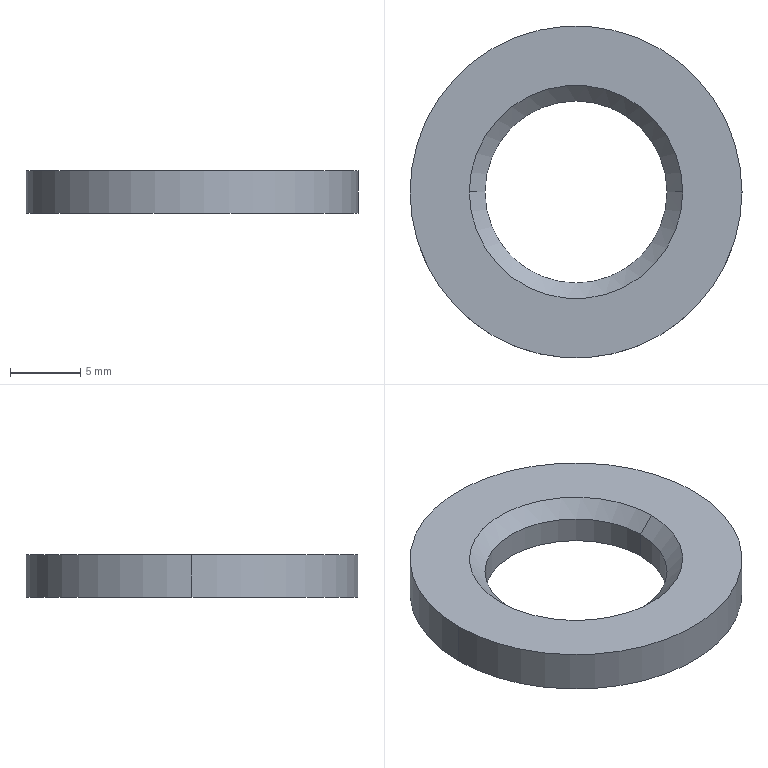Part | SolidWorks | 1 solid | 8 faces | box 23.7 x 23.7 x 3 mm | volume 898.415 mm3 | cylinder 4 | cone 2 | plane 2 | commonest cylinder face diameters 13 x2 23.7 x2
STEP:
#1=CARTESIAN_POINT('',(6.5,0.,1.885));
#2=VERTEX_POINT('',#1);
#3=CARTESIAN_POINT('',(-6.5,0.,1.885));
#4=VERTEX_POINT('',#3);
#5=CARTESIAN_POINT('',(0.,0.,1.885));
#6=DIRECTION('',(0.,0.,-1.));
#7=DIRECTION('',(1.,0.,0.));
#8=AXIS2_PLACEMENT_3D('',#5,#6,#7);
#9=CIRCLE('',#8,6.5);
#10=EDGE_CURVE('',#2,#4,#9,.T.);
#11=ORIENTED_EDGE('',*,*,#10,.T.);
#12=CARTESIAN_POINT('',(-7.615,0.,3.));
#13=VERTEX_POINT('',#12);
#14=CARTESIAN_POINT('',(-7.615,0.,3.));
#15=DIRECTION('',(-0.7071,0.,0.7071));
#16=VECTOR('',#15,1000.);
#17=LINE('',#14,#16);
#18=EDGE_CURVE('',#4,#13,#17,.T.);
#19=ORIENTED_EDGE('',*,*,#18,.T.);
#20=CARTESIAN_POINT('',(7.615,0.,3.));
#21=VERTEX_POINT('',#20);
#22=CARTESIAN_POINT('',(0.,0.,3.));
#23=DIRECTION('',(0.,0.,1.));
#24=DIRECTION('',(1.,0.,0.));
#25=AXIS2_PLACEMENT_3D('',#22,#23,#24);
#26=CIRCLE('',#25,7.615);
#27=EDGE_CURVE('',#13,#21,#26,.T.);
#28=ORIENTED_EDGE('',*,*,#27,.T.);
#29=CARTESIAN_POINT('',(7.615,0.,3.));
#30=DIRECTION('',(0.7071,0.,0.7071));
#31=VECTOR('',#30,1000.);
#32=LINE('',#29,#31);
#33=EDGE_CURVE('',#2,#21,#32,.T.);
#34=ORIENTED_EDGE('',*,*,#33,.F.);
#35=EDGE_LOOP('',(#11,#19,#28,#34));
#36=FACE_OUTER_BOUND('',#35,.T.);
#37=CARTESIAN_POINT('',(0.,0.,3.));
#38=DIRECTION('',(0.,0.,1.));
#39=DIRECTION('',(1.,0.,0.));
#40=AXIS2_PLACEMENT_3D('',#37,#38,#39);
#41=CONICAL_SURFACE('',#40,7.615,0.7854);
#42=ADVANCED_FACE('',(#36),#41,.F.);
#43=ORIENTED_EDGE('',*,*,#10,.F.);
#44=CARTESIAN_POINT('',(6.5,0.,0.));
#45=VERTEX_POINT('',#44);
#46=CARTESIAN_POINT('',(6.5,0.,3.));
#47=DIRECTION('',(0.,0.,-1.));
#48=VECTOR('',#47,1000.);
#49=LINE('',#46,#48);
#50=EDGE_CURVE('',#2,#45,#49,.T.);
#51=ORIENTED_EDGE('',*,*,#50,.T.);
#52=CARTESIAN_POINT('',(-6.5,0.,0.));
#53=VERTEX_POINT('',#52);
#54=CARTESIAN_POINT('',(0.,0.,0.));
#55=DIRECTION('',(0.,0.,1.));
#56=DIRECTION('',(1.,0.,0.));
#57=AXIS2_PLACEMENT_3D('',#54,#55,#56);
#58=CIRCLE('',#57,6.5);
#59=EDGE_CURVE('',#53,#45,#58,.T.);
#60=ORIENTED_EDGE('',*,*,#59,.F.);
#61=CARTESIAN_POINT('',(-6.5,0.,3.));
#62=DIRECTION('',(0.,0.,-1.));
#63=VECTOR('',#62,1000.);
#64=LINE('',#61,#63);
#65=EDGE_CURVE('',#4,#53,#64,.T.);
#66=ORIENTED_EDGE('',*,*,#65,.F.);
#67=EDGE_LOOP('',(#43,#51,#60,#66));
#68=FACE_OUTER_BOUND('',#67,.T.);
#69=CARTESIAN_POINT('',(0.,0.,3.));
#70=DIRECTION('',(0.,0.,-1.));
#71=DIRECTION('',(-1.,0.,0.));
#72=AXIS2_PLACEMENT_3D('',#69,#70,#71);
#73=CYLINDRICAL_SURFACE('',#72,6.5);
#74=ADVANCED_FACE('',(#68),#73,.F.);
#75=CARTESIAN_POINT('',(11.85,0.,3.));
#76=VERTEX_POINT('',#75);
#77=CARTESIAN_POINT('',(-11.85,0.,3.));
#78=VERTEX_POINT('',#77);
#79=CARTESIAN_POINT('',(0.,0.,3.));
#80=DIRECTION('',(0.,0.,1.));
#81=DIRECTION('',(1.,0.,0.));
#82=AXIS2_PLACEMENT_3D('',#79,#80,#81);
#83=CIRCLE('',#82,11.85);
#84=EDGE_CURVE('',#76,#78,#83,.T.);
#85=ORIENTED_EDGE('',*,*,#84,.F.);
#86=CARTESIAN_POINT('',(11.85,0.,0.));
#87=VERTEX_POINT('',#86);
#88=CARTESIAN_POINT('',(11.85,0.,3.));
#89=DIRECTION('',(0.,0.,-1.));
#90=VECTOR('',#89,1000.);
#91=LINE('',#88,#90);
#92=EDGE_CURVE('',#76,#87,#91,.T.);
#93=ORIENTED_EDGE('',*,*,#92,.T.);
#94=CARTESIAN_POINT('',(-11.85,0.,0.));
#95=VERTEX_POINT('',#94);
#96=CARTESIAN_POINT('',(0.,0.,0.));
#97=DIRECTION('',(0.,0.,1.));
#98=DIRECTION('',(1.,0.,0.));
#99=AXIS2_PLACEMENT_3D('',#96,#97,#98);
#100=CIRCLE('',#99,11.85);
#101=EDGE_CURVE('',#87,#95,#100,.T.);
#102=ORIENTED_EDGE('',*,*,#101,.T.);
#103=CARTESIAN_POINT('',(-11.85,0.,3.));
#104=DIRECTION('',(0.,0.,-1.));
#105=VECTOR('',#104,1000.);
#106=LINE('',#103,#105);
#107=EDGE_CURVE('',#78,#95,#106,.T.);
#108=ORIENTED_EDGE('',*,*,#107,.F.);
#109=EDGE_LOOP('',(#85,#93,#102,#108));
#110=FACE_OUTER_BOUND('',#109,.T.);
#111=CARTESIAN_POINT('',(0.,0.,3.));
#112=DIRECTION('',(0.,0.,-1.));
#113=DIRECTION('',(-1.,0.,0.));
#114=AXIS2_PLACEMENT_3D('',#111,#112,#113);
#115=CYLINDRICAL_SURFACE('',#114,11.85);
#116=ADVANCED_FACE('',(#110),#115,.T.);
#117=CARTESIAN_POINT('',(0.,0.,3.));
#118=DIRECTION('',(0.,0.,1.));
#119=DIRECTION('',(1.,0.,0.));
#120=AXIS2_PLACEMENT_3D('',#117,#118,#119);
#121=CIRCLE('',#120,7.615);
#122=EDGE_CURVE('',#21,#13,#121,.T.);
#123=ORIENTED_EDGE('',*,*,#122,.F.);
#124=ORIENTED_EDGE('',*,*,#27,.F.);
#125=EDGE_LOOP('',(#123,#124));
#126=FACE_BOUND('',#125,.T.);
#127=CARTESIAN_POINT('',(0.,0.,3.));
#128=DIRECTION('',(0.,0.,1.));
#129=DIRECTION('',(1.,0.,0.));
#130=AXIS2_PLACEMENT_3D('',#127,#128,#129);
#131=CIRCLE('',#130,11.85);
#132=EDGE_CURVE('',#78,#76,#131,.T.);
#133=ORIENTED_EDGE('',*,*,#132,.T.);
#134=ORIENTED_EDGE('',*,*,#84,.T.);
#135=EDGE_LOOP('',(#133,#134));
#136=FACE_OUTER_BOUND('',#135,.T.);
#137=CARTESIAN_POINT('',(0.,0.,3.));
#138=DIRECTION('',(0.,0.,1.));
#139=DIRECTION('',(1.,0.,0.));
#140=AXIS2_PLACEMENT_3D('',#137,#138,#139);
#141=PLANE('',#140);
#142=ADVANCED_FACE('',(#126,#136),#141,.T.);
#143=CARTESIAN_POINT('',(0.,0.,0.));
#144=DIRECTION('',(0.,0.,1.));
#145=DIRECTION('',(1.,0.,0.));
#146=AXIS2_PLACEMENT_3D('',#143,#144,#145);
#147=CIRCLE('',#146,11.85);
#148=EDGE_CURVE('',#95,#87,#147,.T.);
#149=ORIENTED_EDGE('',*,*,#148,.F.);
#150=ORIENTED_EDGE('',*,*,#101,.F.);
#151=EDGE_LOOP('',(#149,#150));
#152=FACE_OUTER_BOUND('',#151,.T.);
#153=ORIENTED_EDGE('',*,*,#59,.T.);
#154=CARTESIAN_POINT('',(0.,0.,0.));
#155=DIRECTION('',(0.,0.,1.));
#156=DIRECTION('',(1.,0.,0.));
#157=AXIS2_PLACEMENT_3D('',#154,#155,#156);
#158=CIRCLE('',#157,6.5);
#159=EDGE_CURVE('',#45,#53,#158,.T.);
#160=ORIENTED_EDGE('',*,*,#159,.T.);
#161=EDGE_LOOP('',(#153,#160));
#162=FACE_BOUND('',#161,.T.);
#163=CARTESIAN_POINT('',(0.,0.,0.));
#164=DIRECTION('',(0.,0.,1.));
#165=DIRECTION('',(1.,0.,0.));
#166=AXIS2_PLACEMENT_3D('',#163,#164,#165);
#167=PLANE('',#166);
#168=ADVANCED_FACE('',(#152,#162),#167,.F.);
#169=ORIENTED_EDGE('',*,*,#92,.F.);
#170=ORIENTED_EDGE('',*,*,#132,.F.);
#171=ORIENTED_EDGE('',*,*,#107,.T.);
#172=ORIENTED_EDGE('',*,*,#148,.T.);
#173=EDGE_LOOP('',(#169,#170,#171,#172));
#174=FACE_OUTER_BOUND('',#173,.T.);
#175=CARTESIAN_POINT('',(0.,0.,3.));
#176=DIRECTION('',(0.,0.,-1.));
#177=DIRECTION('',(-1.,0.,0.));
#178=AXIS2_PLACEMENT_3D('',#175,#176,#177);
#179=CYLINDRICAL_SURFACE('',#178,11.85);
#180=ADVANCED_FACE('',(#174),#179,.T.);
#181=ORIENTED_EDGE('',*,*,#50,.F.);
#182=CARTESIAN_POINT('',(0.,0.,1.885));
#183=DIRECTION('',(0.,0.,-1.));
#184=DIRECTION('',(1.,0.,0.));
#185=AXIS2_PLACEMENT_3D('',#182,#183,#184);
#186=CIRCLE('',#185,6.5);
#187=EDGE_CURVE('',#4,#2,#186,.T.);
#188=ORIENTED_EDGE('',*,*,#187,.F.);
#189=ORIENTED_EDGE('',*,*,#65,.T.);
#190=ORIENTED_EDGE('',*,*,#159,.F.);
#191=EDGE_LOOP('',(#181,#188,#189,#190));
#192=FACE_OUTER_BOUND('',#191,.T.);
#193=CARTESIAN_POINT('',(0.,0.,3.));
#194=DIRECTION('',(0.,0.,-1.));
#195=DIRECTION('',(-1.,0.,0.));
#196=AXIS2_PLACEMENT_3D('',#193,#194,#195);
#197=CYLINDRICAL_SURFACE('',#196,6.5);
#198=ADVANCED_FACE('',(#192),#197,.F.);
#199=ORIENTED_EDGE('',*,*,#18,.F.);
#200=ORIENTED_EDGE('',*,*,#187,.T.);
#201=ORIENTED_EDGE('',*,*,#33,.T.);
#202=ORIENTED_EDGE('',*,*,#122,.T.);
#203=EDGE_LOOP('',(#199,#200,#201,#202));
#204=FACE_OUTER_BOUND('',#203,.T.);
#205=CARTESIAN_POINT('',(0.,0.,3.));
#206=DIRECTION('',(0.,0.,1.));
#207=DIRECTION('',(1.,0.,0.));
#208=AXIS2_PLACEMENT_3D('',#205,#206,#207);
#209=CONICAL_SURFACE('',#208,7.615,0.7854);
#210=ADVANCED_FACE('',(#204),#209,.F.);
#211=CLOSED_SHELL('',(#42,#74,#116,#142,#168,#180,#198,#210));
#212=MANIFOLD_SOLID_BREP('',#211);
#213=CARTESIAN_POINT('',(0.,0.,0.));
#214=DIRECTION('',(0.,0.,1.));
#215=DIRECTION('',(1.,0.,0.));
#216=AXIS2_PLACEMENT_3D('',#213,#214,#215);
#217=(LENGTH_UNIT()NAMED_UNIT(*)SI_UNIT(.MILLI.,.METRE.));
#218=UNCERTAINTY_MEASURE_WITH_UNIT(LENGTH_MEASURE(0.00001),#217,'','');
#219=(NAMED_UNIT(*)PLANE_ANGLE_UNIT()SI_UNIT($,.RADIAN.));
#220=(NAMED_UNIT(*)SI_UNIT($,.STERADIAN.)SOLID_ANGLE_UNIT());
#221=(GEOMETRIC_REPRESENTATION_CONTEXT(3)GLOBAL_UNCERTAINTY_ASSIGNED_CONTEXT((#218))GLOBAL_UNIT_ASSIGNED_CONTEXT((#217,#219,#220))REPRESENTATION_CONTEXT('',''));
#222=ADVANCED_BREP_SHAPE_REPRESENTATION('',(#212,#216),#221);